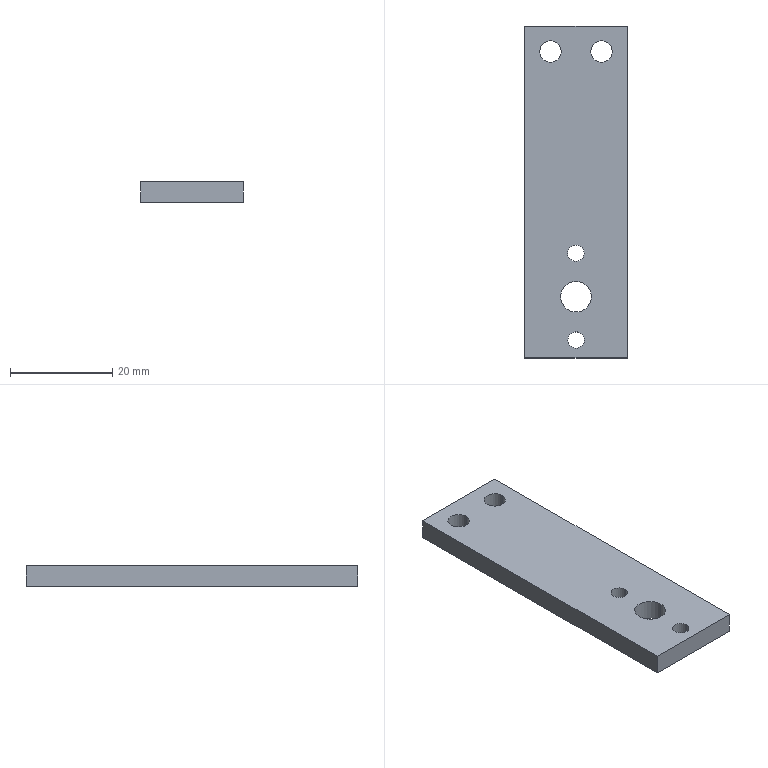Part | SolidWorks | features Extrusion 1 | 1 solid | 16 faces | box 20 x 65 x 4 mm | volume 4912 mm3 | cylinder 10 | plane 6 | commonest cylinder face diameters 3.2 x4 4.2 x4 6 x2
STEP:
#1=CARTESIAN_POINT('',(-1.586,-29.,4.));
#2=VERTEX_POINT('',#1);
#3=CARTESIAN_POINT('',(1.614,-29.,4.));
#4=VERTEX_POINT('',#3);
#5=CARTESIAN_POINT('',(0.01401,-29.,4.));
#6=DIRECTION('',(0.,0.,1.));
#7=DIRECTION('',(1.,0.,0.));
#8=AXIS2_PLACEMENT_3D('',#5,#6,#7);
#9=CIRCLE('',#8,1.6);
#10=EDGE_CURVE('',#2,#4,#9,.T.);
#11=ORIENTED_EDGE('',*,*,#10,.T.);
#12=CARTESIAN_POINT('',(1.614,-29.,0.));
#13=VERTEX_POINT('',#12);
#14=CARTESIAN_POINT('',(1.614,-29.,4.));
#15=DIRECTION('',(0.,0.,-1.));
#16=VECTOR('',#15,1000.);
#17=LINE('',#14,#16);
#18=EDGE_CURVE('',#4,#13,#17,.T.);
#19=ORIENTED_EDGE('',*,*,#18,.T.);
#20=CARTESIAN_POINT('',(-1.586,-29.,0.));
#21=VERTEX_POINT('',#20);
#22=CARTESIAN_POINT('',(0.01401,-29.,0.));
#23=DIRECTION('',(0.,0.,1.));
#24=DIRECTION('',(1.,0.,0.));
#25=AXIS2_PLACEMENT_3D('',#22,#23,#24);
#26=CIRCLE('',#25,1.6);
#27=EDGE_CURVE('',#21,#13,#26,.T.);
#28=ORIENTED_EDGE('',*,*,#27,.F.);
#29=CARTESIAN_POINT('',(-1.586,-29.,4.));
#30=DIRECTION('',(0.,0.,-1.));
#31=VECTOR('',#30,1000.);
#32=LINE('',#29,#31);
#33=EDGE_CURVE('',#2,#21,#32,.T.);
#34=ORIENTED_EDGE('',*,*,#33,.F.);
#35=EDGE_LOOP('',(#11,#19,#28,#34));
#36=FACE_OUTER_BOUND('',#35,.T.);
#37=CARTESIAN_POINT('',(0.01401,-29.,4.));
#38=DIRECTION('',(0.,0.,-1.));
#39=DIRECTION('',(-1.,0.,0.));
#40=AXIS2_PLACEMENT_3D('',#37,#38,#39);
#41=CYLINDRICAL_SURFACE('',#40,1.6);
#42=ADVANCED_FACE('',(#36),#41,.F.);
#43=CARTESIAN_POINT('',(-1.614,-12.,4.));
#44=VERTEX_POINT('',#43);
#45=CARTESIAN_POINT('',(1.586,-12.,4.));
#46=VERTEX_POINT('',#45);
#47=CARTESIAN_POINT('',(-0.01401,-12.,4.));
#48=DIRECTION('',(0.,0.,1.));
#49=DIRECTION('',(1.,0.,0.));
#50=AXIS2_PLACEMENT_3D('',#47,#48,#49);
#51=CIRCLE('',#50,1.6);
#52=EDGE_CURVE('',#44,#46,#51,.T.);
#53=ORIENTED_EDGE('',*,*,#52,.T.);
#54=CARTESIAN_POINT('',(1.586,-12.,0.));
#55=VERTEX_POINT('',#54);
#56=CARTESIAN_POINT('',(1.586,-12.,4.));
#57=DIRECTION('',(0.,0.,-1.));
#58=VECTOR('',#57,1000.);
#59=LINE('',#56,#58);
#60=EDGE_CURVE('',#46,#55,#59,.T.);
#61=ORIENTED_EDGE('',*,*,#60,.T.);
#62=CARTESIAN_POINT('',(-1.614,-12.,0.));
#63=VERTEX_POINT('',#62);
#64=CARTESIAN_POINT('',(-0.01401,-12.,0.));
#65=DIRECTION('',(0.,0.,1.));
#66=DIRECTION('',(1.,0.,0.));
#67=AXIS2_PLACEMENT_3D('',#64,#65,#66);
#68=CIRCLE('',#67,1.6);
#69=EDGE_CURVE('',#63,#55,#68,.T.);
#70=ORIENTED_EDGE('',*,*,#69,.F.);
#71=CARTESIAN_POINT('',(-1.614,-12.,4.));
#72=DIRECTION('',(0.,0.,-1.));
#73=VECTOR('',#72,1000.);
#74=LINE('',#71,#73);
#75=EDGE_CURVE('',#44,#63,#74,.T.);
#76=ORIENTED_EDGE('',*,*,#75,.F.);
#77=EDGE_LOOP('',(#53,#61,#70,#76));
#78=FACE_OUTER_BOUND('',#77,.T.);
#79=CARTESIAN_POINT('',(-0.01401,-12.,4.));
#80=DIRECTION('',(0.,0.,-1.));
#81=DIRECTION('',(-1.,0.,0.));
#82=AXIS2_PLACEMENT_3D('',#79,#80,#81);
#83=CYLINDRICAL_SURFACE('',#82,1.6);
#84=ADVANCED_FACE('',(#78),#83,.F.);
#85=CARTESIAN_POINT('',(-3.,-20.5,4.));
#86=VERTEX_POINT('',#85);
#87=CARTESIAN_POINT('',(3.,-20.5,4.));
#88=VERTEX_POINT('',#87);
#89=CARTESIAN_POINT('',(0.,-20.5,4.));
#90=DIRECTION('',(0.,0.,1.));
#91=DIRECTION('',(1.,0.,0.));
#92=AXIS2_PLACEMENT_3D('',#89,#90,#91);
#93=CIRCLE('',#92,3.);
#94=EDGE_CURVE('',#86,#88,#93,.T.);
#95=ORIENTED_EDGE('',*,*,#94,.T.);
#96=CARTESIAN_POINT('',(3.,-20.5,0.));
#97=VERTEX_POINT('',#96);
#98=CARTESIAN_POINT('',(3.,-20.5,4.));
#99=DIRECTION('',(0.,0.,-1.));
#100=VECTOR('',#99,1000.);
#101=LINE('',#98,#100);
#102=EDGE_CURVE('',#88,#97,#101,.T.);
#103=ORIENTED_EDGE('',*,*,#102,.T.);
#104=CARTESIAN_POINT('',(-3.,-20.5,0.));
#105=VERTEX_POINT('',#104);
#106=CARTESIAN_POINT('',(0.,-20.5,0.));
#107=DIRECTION('',(0.,0.,1.));
#108=DIRECTION('',(1.,0.,0.));
#109=AXIS2_PLACEMENT_3D('',#106,#107,#108);
#110=CIRCLE('',#109,3.);
#111=EDGE_CURVE('',#105,#97,#110,.T.);
#112=ORIENTED_EDGE('',*,*,#111,.F.);
#113=CARTESIAN_POINT('',(-3.,-20.5,4.));
#114=DIRECTION('',(0.,0.,-1.));
#115=VECTOR('',#114,1000.);
#116=LINE('',#113,#115);
#117=EDGE_CURVE('',#86,#105,#116,.T.);
#118=ORIENTED_EDGE('',*,*,#117,.F.);
#119=EDGE_LOOP('',(#95,#103,#112,#118));
#120=FACE_OUTER_BOUND('',#119,.T.);
#121=CARTESIAN_POINT('',(0.,-20.5,4.));
#122=DIRECTION('',(0.,0.,-1.));
#123=DIRECTION('',(-1.,0.,0.));
#124=AXIS2_PLACEMENT_3D('',#121,#122,#123);
#125=CYLINDRICAL_SURFACE('',#124,3.);
#126=ADVANCED_FACE('',(#120),#125,.F.);
#127=CARTESIAN_POINT('',(2.9,27.5,4.));
#128=VERTEX_POINT('',#127);
#129=CARTESIAN_POINT('',(7.1,27.5,4.));
#130=VERTEX_POINT('',#129);
#131=CARTESIAN_POINT('',(5.,27.5,4.));
#132=DIRECTION('',(0.,0.,1.));
#133=DIRECTION('',(1.,0.,0.));
#134=AXIS2_PLACEMENT_3D('',#131,#132,#133);
#135=CIRCLE('',#134,2.1);
#136=EDGE_CURVE('',#128,#130,#135,.T.);
#137=ORIENTED_EDGE('',*,*,#136,.T.);
#138=CARTESIAN_POINT('',(7.1,27.5,0.));
#139=VERTEX_POINT('',#138);
#140=CARTESIAN_POINT('',(7.1,27.5,4.));
#141=DIRECTION('',(0.,0.,-1.));
#142=VECTOR('',#141,1000.);
#143=LINE('',#140,#142);
#144=EDGE_CURVE('',#130,#139,#143,.T.);
#145=ORIENTED_EDGE('',*,*,#144,.T.);
#146=CARTESIAN_POINT('',(2.9,27.5,0.));
#147=VERTEX_POINT('',#146);
#148=CARTESIAN_POINT('',(5.,27.5,0.));
#149=DIRECTION('',(0.,0.,1.));
#150=DIRECTION('',(1.,0.,0.));
#151=AXIS2_PLACEMENT_3D('',#148,#149,#150);
#152=CIRCLE('',#151,2.1);
#153=EDGE_CURVE('',#147,#139,#152,.T.);
#154=ORIENTED_EDGE('',*,*,#153,.F.);
#155=CARTESIAN_POINT('',(2.9,27.5,4.));
#156=DIRECTION('',(0.,0.,-1.));
#157=VECTOR('',#156,1000.);
#158=LINE('',#155,#157);
#159=EDGE_CURVE('',#128,#147,#158,.T.);
#160=ORIENTED_EDGE('',*,*,#159,.F.);
#161=EDGE_LOOP('',(#137,#145,#154,#160));
#162=FACE_OUTER_BOUND('',#161,.T.);
#163=CARTESIAN_POINT('',(5.,27.5,4.));
#164=DIRECTION('',(0.,0.,-1.));
#165=DIRECTION('',(-1.,0.,0.));
#166=AXIS2_PLACEMENT_3D('',#163,#164,#165);
#167=CYLINDRICAL_SURFACE('',#166,2.1);
#168=ADVANCED_FACE('',(#162),#167,.F.);
#169=CARTESIAN_POINT('',(-7.1,27.5,4.));
#170=VERTEX_POINT('',#169);
#171=CARTESIAN_POINT('',(-2.9,27.5,4.));
#172=VERTEX_POINT('',#171);
#173=CARTESIAN_POINT('',(-5.,27.5,4.));
#174=DIRECTION('',(0.,0.,1.));
#175=DIRECTION('',(1.,0.,0.));
#176=AXIS2_PLACEMENT_3D('',#173,#174,#175);
#177=CIRCLE('',#176,2.1);
#178=EDGE_CURVE('',#170,#172,#177,.T.);
#179=ORIENTED_EDGE('',*,*,#178,.T.);
#180=CARTESIAN_POINT('',(-2.9,27.5,0.));
#181=VERTEX_POINT('',#180);
#182=CARTESIAN_POINT('',(-2.9,27.5,4.));
#183=DIRECTION('',(0.,0.,-1.));
#184=VECTOR('',#183,1000.);
#185=LINE('',#182,#184);
#186=EDGE_CURVE('',#172,#181,#185,.T.);
#187=ORIENTED_EDGE('',*,*,#186,.T.);
#188=CARTESIAN_POINT('',(-7.1,27.5,0.));
#189=VERTEX_POINT('',#188);
#190=CARTESIAN_POINT('',(-5.,27.5,0.));
#191=DIRECTION('',(0.,0.,1.));
#192=DIRECTION('',(1.,0.,0.));
#193=AXIS2_PLACEMENT_3D('',#190,#191,#192);
#194=CIRCLE('',#193,2.1);
#195=EDGE_CURVE('',#189,#181,#194,.T.);
#196=ORIENTED_EDGE('',*,*,#195,.F.);
#197=CARTESIAN_POINT('',(-7.1,27.5,4.));
#198=DIRECTION('',(0.,0.,-1.));
#199=VECTOR('',#198,1000.);
#200=LINE('',#197,#199);
#201=EDGE_CURVE('',#170,#189,#200,.T.);
#202=ORIENTED_EDGE('',*,*,#201,.F.);
#203=EDGE_LOOP('',(#179,#187,#196,#202));
#204=FACE_OUTER_BOUND('',#203,.T.);
#205=CARTESIAN_POINT('',(-5.,27.5,4.));
#206=DIRECTION('',(0.,0.,-1.));
#207=DIRECTION('',(-1.,0.,0.));
#208=AXIS2_PLACEMENT_3D('',#205,#206,#207);
#209=CYLINDRICAL_SURFACE('',#208,2.1);
#210=ADVANCED_FACE('',(#204),#209,.F.);
#211=CARTESIAN_POINT('',(10.,-32.5,4.));
#212=VERTEX_POINT('',#211);
#213=CARTESIAN_POINT('',(10.,32.5,4.));
#214=VERTEX_POINT('',#213);
#215=CARTESIAN_POINT('',(10.,-32.5,4.));
#216=DIRECTION('',(0.,1.,0.));
#217=VECTOR('',#216,1000.);
#218=LINE('',#215,#217);
#219=EDGE_CURVE('',#212,#214,#218,.T.);
#220=ORIENTED_EDGE('',*,*,#219,.T.);
#221=CARTESIAN_POINT('',(-10.,32.5,4.));
#222=VERTEX_POINT('',#221);
#223=CARTESIAN_POINT('',(-10.,32.5,4.));
#224=DIRECTION('',(-1.,0.,0.));
#225=VECTOR('',#224,1000.);
#226=LINE('',#223,#225);
#227=EDGE_CURVE('',#214,#222,#226,.T.);
#228=ORIENTED_EDGE('',*,*,#227,.T.);
#229=CARTESIAN_POINT('',(-10.,-32.5,4.));
#230=VERTEX_POINT('',#229);
#231=CARTESIAN_POINT('',(-10.,-32.5,4.));
#232=DIRECTION('',(0.,-1.,0.));
#233=VECTOR('',#232,1000.);
#234=LINE('',#231,#233);
#235=EDGE_CURVE('',#222,#230,#234,.T.);
#236=ORIENTED_EDGE('',*,*,#235,.T.);
#237=CARTESIAN_POINT('',(-10.,-32.5,4.));
#238=DIRECTION('',(1.,0.,0.));
#239=VECTOR('',#238,1000.);
#240=LINE('',#237,#239);
#241=EDGE_CURVE('',#230,#212,#240,.T.);
#242=ORIENTED_EDGE('',*,*,#241,.T.);
#243=EDGE_LOOP('',(#220,#228,#236,#242));
#244=FACE_OUTER_BOUND('',#243,.T.);
#245=ORIENTED_EDGE('',*,*,#178,.F.);
#246=CARTESIAN_POINT('',(-5.,27.5,4.));
#247=DIRECTION('',(0.,0.,1.));
#248=DIRECTION('',(1.,0.,0.));
#249=AXIS2_PLACEMENT_3D('',#246,#247,#248);
#250=CIRCLE('',#249,2.1);
#251=EDGE_CURVE('',#172,#170,#250,.T.);
#252=ORIENTED_EDGE('',*,*,#251,.F.);
#253=EDGE_LOOP('',(#245,#252));
#254=FACE_BOUND('',#253,.T.);
#255=ORIENTED_EDGE('',*,*,#136,.F.);
#256=CARTESIAN_POINT('',(5.,27.5,4.));
#257=DIRECTION('',(0.,0.,1.));
#258=DIRECTION('',(1.,0.,0.));
#259=AXIS2_PLACEMENT_3D('',#256,#257,#258);
#260=CIRCLE('',#259,2.1);
#261=EDGE_CURVE('',#130,#128,#260,.T.);
#262=ORIENTED_EDGE('',*,*,#261,.F.);
#263=EDGE_LOOP('',(#255,#262));
#264=FACE_BOUND('',#263,.T.);
#265=ORIENTED_EDGE('',*,*,#94,.F.);
#266=CARTESIAN_POINT('',(0.,-20.5,4.));
#267=DIRECTION('',(0.,0.,1.));
#268=DIRECTION('',(1.,0.,0.));
#269=AXIS2_PLACEMENT_3D('',#266,#267,#268);
#270=CIRCLE('',#269,3.);
#271=EDGE_CURVE('',#88,#86,#270,.T.);
#272=ORIENTED_EDGE('',*,*,#271,.F.);
#273=EDGE_LOOP('',(#265,#272));
#274=FACE_BOUND('',#273,.T.);
#275=ORIENTED_EDGE('',*,*,#52,.F.);
#276=CARTESIAN_POINT('',(-0.01401,-12.,4.));
#277=DIRECTION('',(0.,0.,1.));
#278=DIRECTION('',(1.,0.,0.));
#279=AXIS2_PLACEMENT_3D('',#276,#277,#278);
#280=CIRCLE('',#279,1.6);
#281=EDGE_CURVE('',#46,#44,#280,.T.);
#282=ORIENTED_EDGE('',*,*,#281,.F.);
#283=EDGE_LOOP('',(#275,#282));
#284=FACE_BOUND('',#283,.T.);
#285=ORIENTED_EDGE('',*,*,#10,.F.);
#286=CARTESIAN_POINT('',(0.01401,-29.,4.));
#287=DIRECTION('',(0.,0.,1.));
#288=DIRECTION('',(1.,0.,0.));
#289=AXIS2_PLACEMENT_3D('',#286,#287,#288);
#290=CIRCLE('',#289,1.6);
#291=EDGE_CURVE('',#4,#2,#290,.T.);
#292=ORIENTED_EDGE('',*,*,#291,.F.);
#293=EDGE_LOOP('',(#285,#292));
#294=FACE_BOUND('',#293,.T.);
#295=CARTESIAN_POINT('',(0.,0.,4.));
#296=DIRECTION('',(0.,0.,-1.));
#297=DIRECTION('',(-1.,0.,0.));
#298=AXIS2_PLACEMENT_3D('',#295,#296,#297);
#299=PLANE('',#298);
#300=ADVANCED_FACE('',(#244,#254,#264,#274,#284,#294),#299,.F.);
#301=ORIENTED_EDGE('',*,*,#69,.T.);
#302=CARTESIAN_POINT('',(-0.01401,-12.,0.));
#303=DIRECTION('',(0.,0.,1.));
#304=DIRECTION('',(1.,0.,0.));
#305=AXIS2_PLACEMENT_3D('',#302,#303,#304);
#306=CIRCLE('',#305,1.6);
#307=EDGE_CURVE('',#55,#63,#306,.T.);
#308=ORIENTED_EDGE('',*,*,#307,.T.);
#309=EDGE_LOOP('',(#301,#308));
#310=FACE_BOUND('',#309,.T.);
#311=ORIENTED_EDGE('',*,*,#153,.T.);
#312=CARTESIAN_POINT('',(5.,27.5,0.));
#313=DIRECTION('',(0.,0.,1.));
#314=DIRECTION('',(1.,0.,0.));
#315=AXIS2_PLACEMENT_3D('',#312,#313,#314);
#316=CIRCLE('',#315,2.1);
#317=EDGE_CURVE('',#139,#147,#316,.T.);
#318=ORIENTED_EDGE('',*,*,#317,.T.);
#319=EDGE_LOOP('',(#311,#318));
#320=FACE_BOUND('',#319,.T.);
#321=CARTESIAN_POINT('',(10.,-32.5,0.));
#322=VERTEX_POINT('',#321);
#323=CARTESIAN_POINT('',(10.,32.5,0.));
#324=VERTEX_POINT('',#323);
#325=CARTESIAN_POINT('',(10.,-32.5,0.));
#326=DIRECTION('',(0.,1.,0.));
#327=VECTOR('',#326,1000.);
#328=LINE('',#325,#327);
#329=EDGE_CURVE('',#322,#324,#328,.T.);
#330=ORIENTED_EDGE('',*,*,#329,.F.);
#331=CARTESIAN_POINT('',(-10.,-32.5,0.));
#332=VERTEX_POINT('',#331);
#333=CARTESIAN_POINT('',(-10.,-32.5,0.));
#334=DIRECTION('',(1.,0.,0.));
#335=VECTOR('',#334,1000.);
#336=LINE('',#333,#335);
#337=EDGE_CURVE('',#332,#322,#336,.T.);
#338=ORIENTED_EDGE('',*,*,#337,.F.);
#339=CARTESIAN_POINT('',(-10.,32.5,0.));
#340=VERTEX_POINT('',#339);
#341=CARTESIAN_POINT('',(-10.,-32.5,0.));
#342=DIRECTION('',(0.,-1.,0.));
#343=VECTOR('',#342,1000.);
#344=LINE('',#341,#343);
#345=EDGE_CURVE('',#340,#332,#344,.T.);
#346=ORIENTED_EDGE('',*,*,#345,.F.);
#347=CARTESIAN_POINT('',(-10.,32.5,0.));
#348=DIRECTION('',(-1.,0.,0.));
#349=VECTOR('',#348,1000.);
#350=LINE('',#347,#349);
#351=EDGE_CURVE('',#324,#340,#350,.T.);
#352=ORIENTED_EDGE('',*,*,#351,.F.);
#353=EDGE_LOOP('',(#330,#338,#346,#352));
#354=FACE_OUTER_BOUND('',#353,.T.);
#355=ORIENTED_EDGE('',*,*,#195,.T.);
#356=CARTESIAN_POINT('',(-5.,27.5,0.));
#357=DIRECTION('',(0.,0.,1.));
#358=DIRECTION('',(1.,0.,0.));
#359=AXIS2_PLACEMENT_3D('',#356,#357,#358);
#360=CIRCLE('',#359,2.1);
#361=EDGE_CURVE('',#181,#189,#360,.T.);
#362=ORIENTED_EDGE('',*,*,#361,.T.);
#363=EDGE_LOOP('',(#355,#362));
#364=FACE_BOUND('',#363,.T.);
#365=ORIENTED_EDGE('',*,*,#111,.T.);
#366=CARTESIAN_POINT('',(0.,-20.5,0.));
#367=DIRECTION('',(0.,0.,1.));
#368=DIRECTION('',(1.,0.,0.));
#369=AXIS2_PLACEMENT_3D('',#366,#367,#368);
#370=CIRCLE('',#369,3.);
#371=EDGE_CURVE('',#97,#105,#370,.T.);
#372=ORIENTED_EDGE('',*,*,#371,.T.);
#373=EDGE_LOOP('',(#365,#372));
#374=FACE_BOUND('',#373,.T.);
#375=ORIENTED_EDGE('',*,*,#27,.T.);
#376=CARTESIAN_POINT('',(0.01401,-29.,0.));
#377=DIRECTION('',(0.,0.,1.));
#378=DIRECTION('',(1.,0.,0.));
#379=AXIS2_PLACEMENT_3D('',#376,#377,#378);
#380=CIRCLE('',#379,1.6);
#381=EDGE_CURVE('',#13,#21,#380,.T.);
#382=ORIENTED_EDGE('',*,*,#381,.T.);
#383=EDGE_LOOP('',(#375,#382));
#384=FACE_BOUND('',#383,.T.);
#385=CARTESIAN_POINT('',(0.,0.,0.));
#386=DIRECTION('',(0.,0.,-1.));
#387=DIRECTION('',(-1.,0.,0.));
#388=AXIS2_PLACEMENT_3D('',#385,#386,#387);
#389=PLANE('',#388);
#390=ADVANCED_FACE('',(#310,#320,#354,#364,#374,#384),#389,.T.);
#391=ORIENTED_EDGE('',*,*,#329,.T.);
#392=CARTESIAN_POINT('',(10.,32.5,4.));
#393=DIRECTION('',(0.,0.,-1.));
#394=VECTOR('',#393,1000.);
#395=LINE('',#392,#394);
#396=EDGE_CURVE('',#214,#324,#395,.T.);
#397=ORIENTED_EDGE('',*,*,#396,.F.);
#398=ORIENTED_EDGE('',*,*,#219,.F.);
#399=CARTESIAN_POINT('',(10.,-32.5,4.));
#400=DIRECTION('',(0.,0.,-1.));
#401=VECTOR('',#400,1000.);
#402=LINE('',#399,#401);
#403=EDGE_CURVE('',#212,#322,#402,.T.);
#404=ORIENTED_EDGE('',*,*,#403,.T.);
#405=EDGE_LOOP('',(#391,#397,#398,#404));
#406=FACE_OUTER_BOUND('',#405,.T.);
#407=CARTESIAN_POINT('',(10.,-32.5,4.));
#408=DIRECTION('',(-1.,0.,0.));
#409=DIRECTION('',(0.,0.,1.));
#410=AXIS2_PLACEMENT_3D('',#407,#408,#409);
#411=PLANE('',#410);
#412=ADVANCED_FACE('',(#406),#411,.F.);
#413=ORIENTED_EDGE('',*,*,#351,.T.);
#414=CARTESIAN_POINT('',(-10.,32.5,4.));
#415=DIRECTION('',(0.,0.,-1.));
#416=VECTOR('',#415,1000.);
#417=LINE('',#414,#416);
#418=EDGE_CURVE('',#222,#340,#417,.T.);
#419=ORIENTED_EDGE('',*,*,#418,.F.);
#420=ORIENTED_EDGE('',*,*,#227,.F.);
#421=ORIENTED_EDGE('',*,*,#396,.T.);
#422=EDGE_LOOP('',(#413,#419,#420,#421));
#423=FACE_OUTER_BOUND('',#422,.T.);
#424=CARTESIAN_POINT('',(-10.,32.5,4.));
#425=DIRECTION('',(0.,-1.,0.));
#426=DIRECTION('',(0.,0.,-1.));
#427=AXIS2_PLACEMENT_3D('',#424,#425,#426);
#428=PLANE('',#427);
#429=ADVANCED_FACE('',(#423),#428,.F.);
#430=ORIENTED_EDGE('',*,*,#345,.T.);
#431=CARTESIAN_POINT('',(-10.,-32.5,4.));
#432=DIRECTION('',(0.,0.,-1.));
#433=VECTOR('',#432,1000.);
#434=LINE('',#431,#433);
#435=EDGE_CURVE('',#230,#332,#434,.T.);
#436=ORIENTED_EDGE('',*,*,#435,.F.);
#437=ORIENTED_EDGE('',*,*,#235,.F.);
#438=ORIENTED_EDGE('',*,*,#418,.T.);
#439=EDGE_LOOP('',(#430,#436,#437,#438));
#440=FACE_OUTER_BOUND('',#439,.T.);
#441=CARTESIAN_POINT('',(-10.,-32.5,4.));
#442=DIRECTION('',(1.,0.,0.));
#443=DIRECTION('',(0.,0.,-1.));
#444=AXIS2_PLACEMENT_3D('',#441,#442,#443);
#445=PLANE('',#444);
#446=ADVANCED_FACE('',(#440),#445,.F.);
#447=ORIENTED_EDGE('',*,*,#337,.T.);
#448=ORIENTED_EDGE('',*,*,#403,.F.);
#449=ORIENTED_EDGE('',*,*,#241,.F.);
#450=ORIENTED_EDGE('',*,*,#435,.T.);
#451=EDGE_LOOP('',(#447,#448,#449,#450));
#452=FACE_OUTER_BOUND('',#451,.T.);
#453=CARTESIAN_POINT('',(-10.,-32.5,4.));
#454=DIRECTION('',(0.,1.,0.));
#455=DIRECTION('',(0.,0.,1.));
#456=AXIS2_PLACEMENT_3D('',#453,#454,#455);
#457=PLANE('',#456);
#458=ADVANCED_FACE('',(#452),#457,.F.);
#459=ORIENTED_EDGE('',*,*,#186,.F.);
#460=ORIENTED_EDGE('',*,*,#251,.T.);
#461=ORIENTED_EDGE('',*,*,#201,.T.);
#462=ORIENTED_EDGE('',*,*,#361,.F.);
#463=EDGE_LOOP('',(#459,#460,#461,#462));
#464=FACE_OUTER_BOUND('',#463,.T.);
#465=CARTESIAN_POINT('',(-5.,27.5,4.));
#466=DIRECTION('',(0.,0.,-1.));
#467=DIRECTION('',(-1.,0.,0.));
#468=AXIS2_PLACEMENT_3D('',#465,#466,#467);
#469=CYLINDRICAL_SURFACE('',#468,2.1);
#470=ADVANCED_FACE('',(#464),#469,.F.);
#471=ORIENTED_EDGE('',*,*,#144,.F.);
#472=ORIENTED_EDGE('',*,*,#261,.T.);
#473=ORIENTED_EDGE('',*,*,#159,.T.);
#474=ORIENTED_EDGE('',*,*,#317,.F.);
#475=EDGE_LOOP('',(#471,#472,#473,#474));
#476=FACE_OUTER_BOUND('',#475,.T.);
#477=CARTESIAN_POINT('',(5.,27.5,4.));
#478=DIRECTION('',(0.,0.,-1.));
#479=DIRECTION('',(-1.,0.,0.));
#480=AXIS2_PLACEMENT_3D('',#477,#478,#479);
#481=CYLINDRICAL_SURFACE('',#480,2.1);
#482=ADVANCED_FACE('',(#476),#481,.F.);
#483=ORIENTED_EDGE('',*,*,#102,.F.);
#484=ORIENTED_EDGE('',*,*,#271,.T.);
#485=ORIENTED_EDGE('',*,*,#117,.T.);
#486=ORIENTED_EDGE('',*,*,#371,.F.);
#487=EDGE_LOOP('',(#483,#484,#485,#486));
#488=FACE_OUTER_BOUND('',#487,.T.);
#489=CARTESIAN_POINT('',(0.,-20.5,4.));
#490=DIRECTION('',(0.,0.,-1.));
#491=DIRECTION('',(-1.,0.,0.));
#492=AXIS2_PLACEMENT_3D('',#489,#490,#491);
#493=CYLINDRICAL_SURFACE('',#492,3.);
#494=ADVANCED_FACE('',(#488),#493,.F.);
#495=ORIENTED_EDGE('',*,*,#60,.F.);
#496=ORIENTED_EDGE('',*,*,#281,.T.);
#497=ORIENTED_EDGE('',*,*,#75,.T.);
#498=ORIENTED_EDGE('',*,*,#307,.F.);
#499=EDGE_LOOP('',(#495,#496,#497,#498));
#500=FACE_OUTER_BOUND('',#499,.T.);
#501=CARTESIAN_POINT('',(-0.01401,-12.,4.));
#502=DIRECTION('',(0.,0.,-1.));
#503=DIRECTION('',(-1.,0.,0.));
#504=AXIS2_PLACEMENT_3D('',#501,#502,#503);
#505=CYLINDRICAL_SURFACE('',#504,1.6);
#506=ADVANCED_FACE('',(#500),#505,.F.);
#507=ORIENTED_EDGE('',*,*,#18,.F.);
#508=ORIENTED_EDGE('',*,*,#291,.T.);
#509=ORIENTED_EDGE('',*,*,#33,.T.);
#510=ORIENTED_EDGE('',*,*,#381,.F.);
#511=EDGE_LOOP('',(#507,#508,#509,#510));
#512=FACE_OUTER_BOUND('',#511,.T.);
#513=CARTESIAN_POINT('',(0.01401,-29.,4.));
#514=DIRECTION('',(0.,0.,-1.));
#515=DIRECTION('',(-1.,0.,0.));
#516=AXIS2_PLACEMENT_3D('',#513,#514,#515);
#517=CYLINDRICAL_SURFACE('',#516,1.6);
#518=ADVANCED_FACE('',(#512),#517,.F.);
#519=CLOSED_SHELL('',(#42,#84,#126,#168,#210,#300,#390,#412,#429,#446,#458,#470,#482,#494,#506,#518));
#520=MANIFOLD_SOLID_BREP('',#519);
#521=CARTESIAN_POINT('',(0.,0.,0.));
#522=DIRECTION('',(0.,0.,1.));
#523=DIRECTION('',(1.,0.,0.));
#524=AXIS2_PLACEMENT_3D('',#521,#522,#523);
#525=(LENGTH_UNIT()NAMED_UNIT(*)SI_UNIT(.MILLI.,.METRE.));
#526=UNCERTAINTY_MEASURE_WITH_UNIT(LENGTH_MEASURE(0.00001),#525,'','');
#527=(NAMED_UNIT(*)PLANE_ANGLE_UNIT()SI_UNIT($,.RADIAN.));
#528=(NAMED_UNIT(*)SI_UNIT($,.STERADIAN.)SOLID_ANGLE_UNIT());
#529=(GEOMETRIC_REPRESENTATION_CONTEXT(3)GLOBAL_UNCERTAINTY_ASSIGNED_CONTEXT((#526))GLOBAL_UNIT_ASSIGNED_CONTEXT((#525,#527,#528))REPRESENTATION_CONTEXT('',''));
#530=ADVANCED_BREP_SHAPE_REPRESENTATION('',(#520,#524),#529);